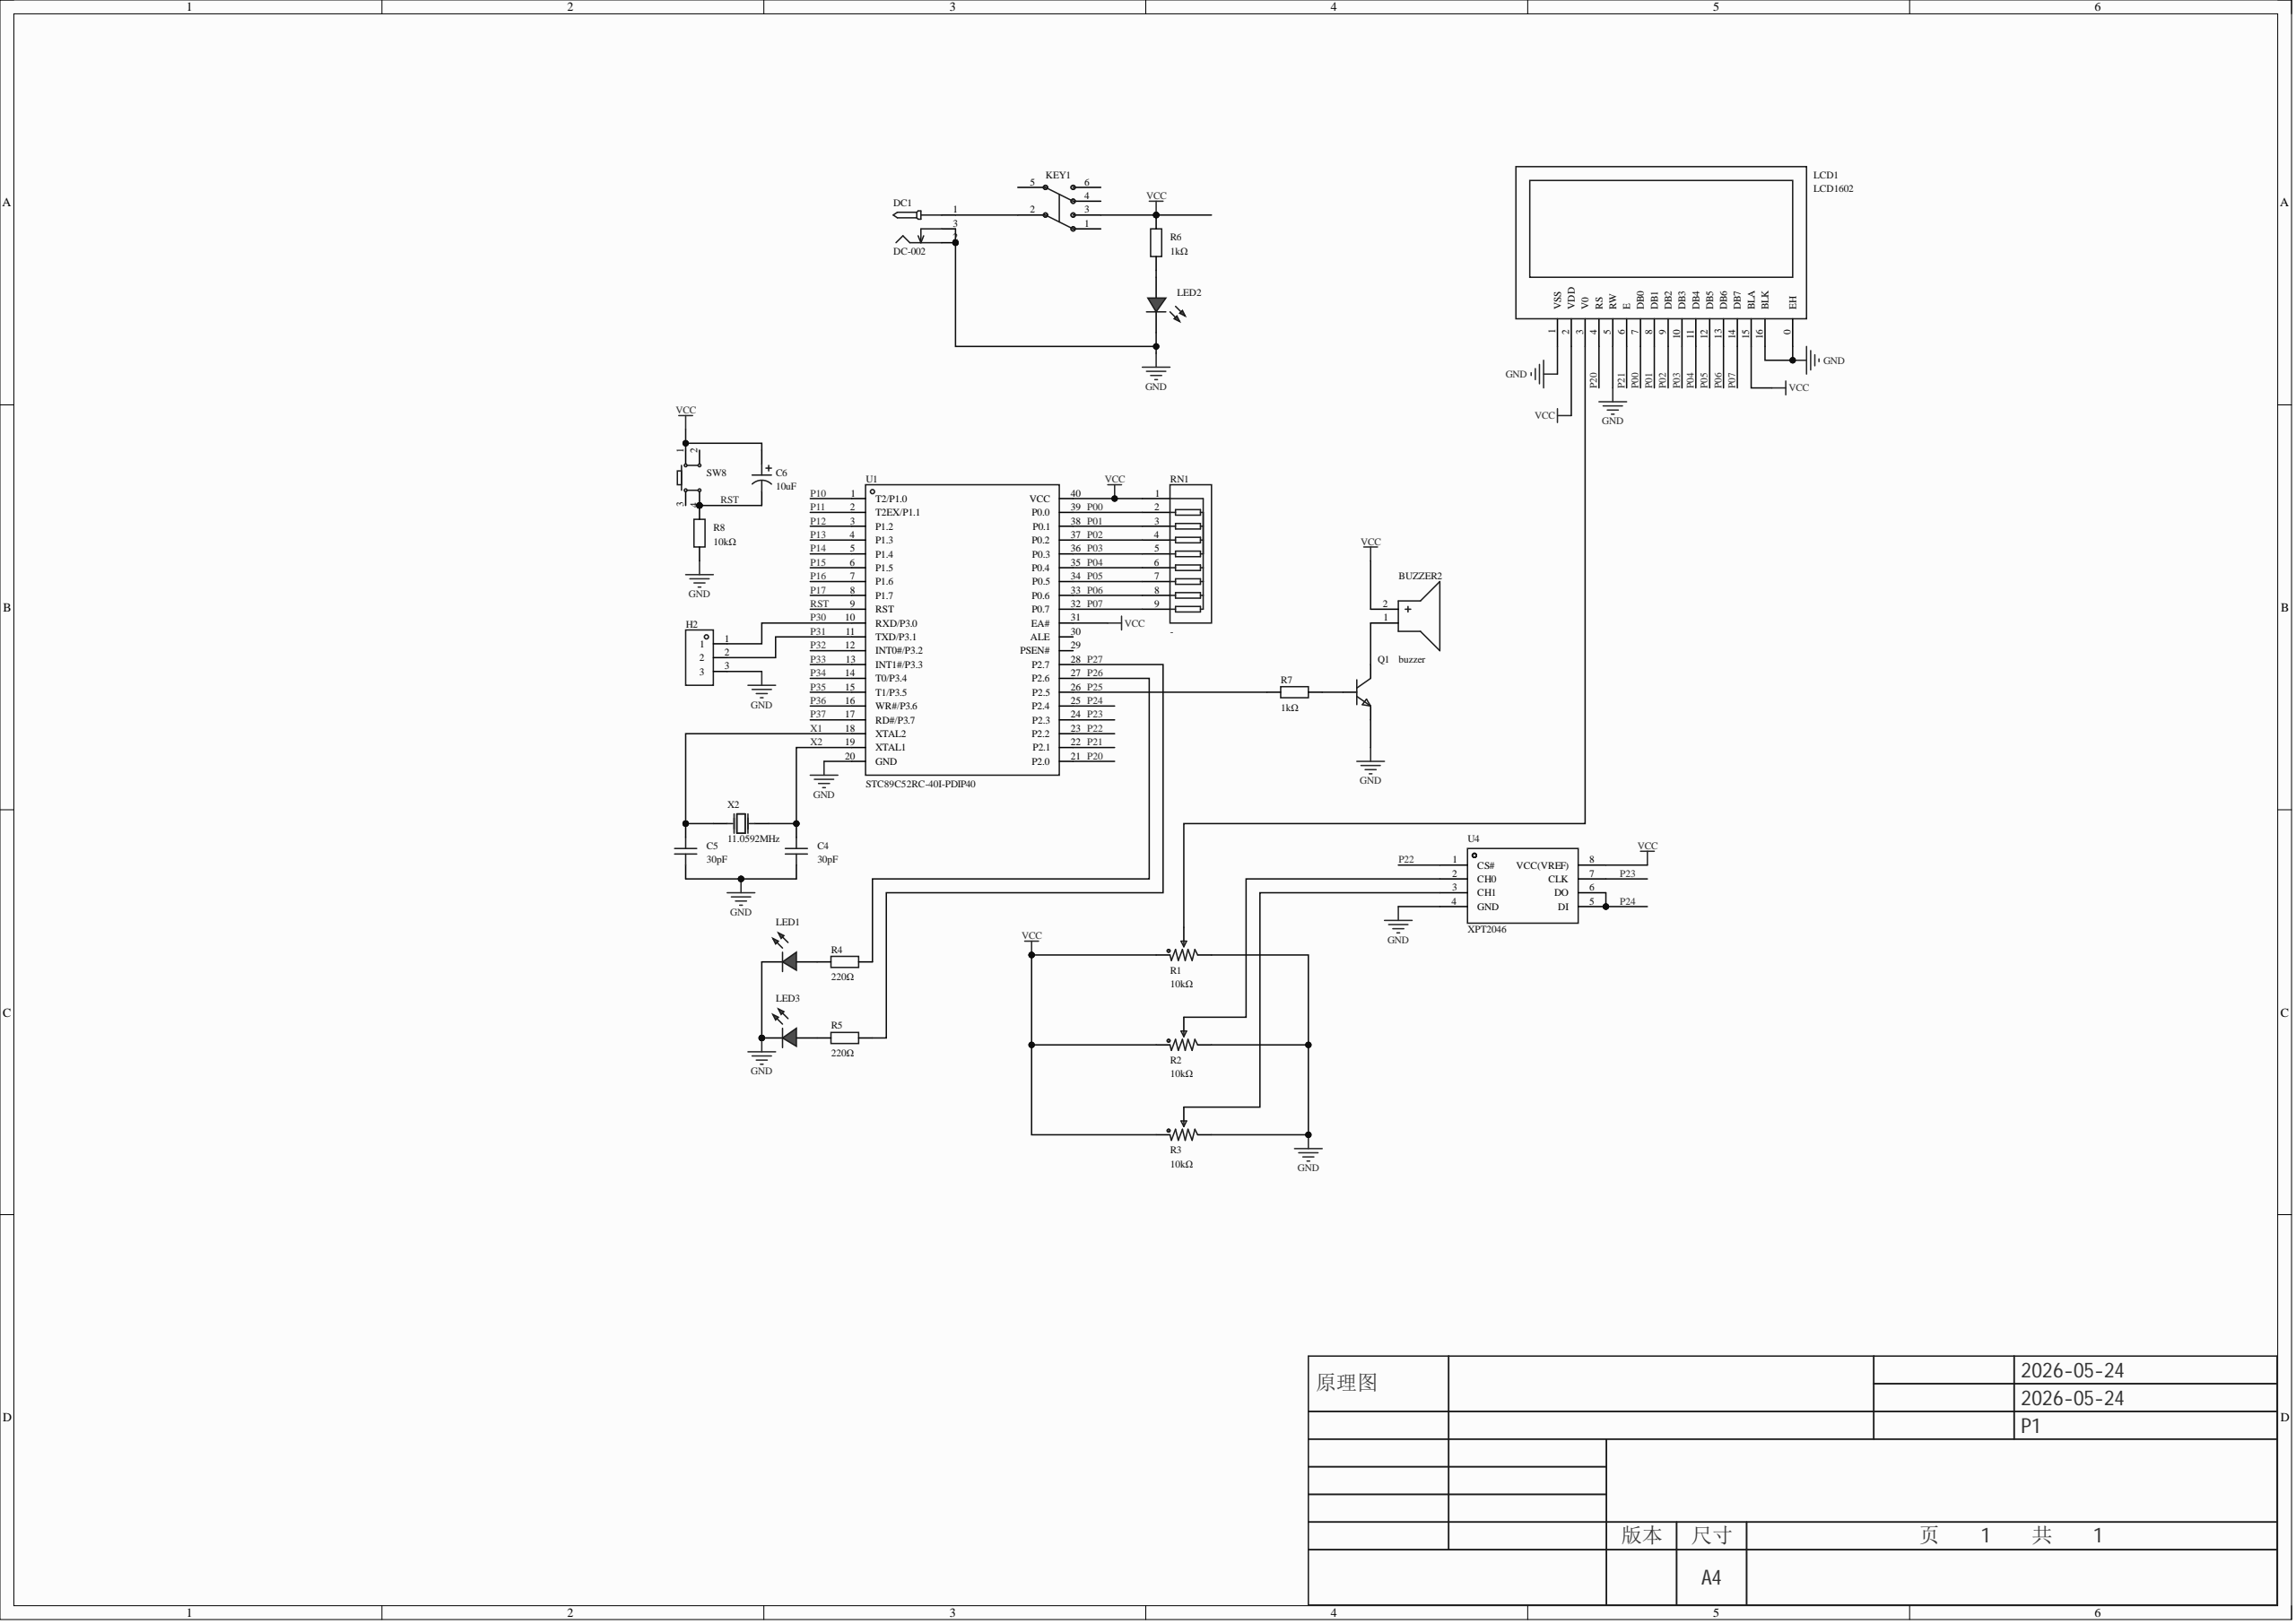Circuit board | Altium Designer | 25 parts | 32 nets
Bill of materials:
Comment,Description,Designator,Footprint,LibRef,Quantity
"buzzer","","BUZZER2","BUZ-TH_BD12.0-P6.00-D0.9-RD","buzzer","1"
"30pF","","C4, C5","CAP-TH_L3.8-W2.5-P2.54-D0.50","C315C300K3G5TA7301","2"
"10uF","","C6","CAP-TH_BD5.0-P2.00-D0.8-FD-10UF50VC110GL","10UF50VC110GL","1"
"DC-002","","DC1","DC-IN-TH_DC-3510","DC-002","1"
"","","H2","HDR-TH_3P-P2.54-V-M","HDR-M_2.54_1x3P","1"
"无自锁开关 8.5×8.5 无声","","KEY1","SW-TH_6P-L8.5-W8.5-P2.54","无自锁开关 8.5×8.5 无声","1"
"LCD1602","","LCD1","LCD1602","HS1602A","1"
"","","LED1, LED2, LED3","LED_TH-3mm","LED_TH-R_3mm","3"
"","","Q1","S8050_TO_92","S8050_TO_NPN","1"
"10kΩ","","R1, R2, R3","RES-ADJ-SMD_RM065-V1","RM065-103(10K)","3"
"220Ω","","R4, R5","Res_1/8W","Res_AXIAL-1/8W","2"
"1kΩ","","R6, R7","Res_1/8W","Res_AXIAL-1/8W","2"
"10kΩ","","R8","Res_1/8W","Res_AXIAL-1/8W","1"
"-","","RN1","RES-ARRAY-TH_9P-P2.54-D1.0","排阻 10 K 5%","1"
"","","SW8","SW-TH_4P-L6.0-W6.0-P4.50-LS6.5","Key_TH_6x6x6","1"
"STC89C52RC-40I-PDIP40","","U1","DIP-40_L52.0-W13.7-P2.54-LS15.2-BL","STC89C52RC-40I-PDIP40","1"
"XPT2046","","U4","DIP-8_L9.7-W6.4-P2.54-LS7.6-BL","ADC0832CCN","1"
"11.059MHz","","X2","OSC-TH_L11.1-W4.7-P4.88","9AC11059302060C3","1"
Netlist (Protel format):
[
BUZZER2
BUZ-TH_BD12.0-P6.00-D0.9-RD
buzzer



]
[
C4
CAP-TH_L3.8-W2.5-P2.54-D0.50
30pF



]
[
C5
CAP-TH_L3.8-W2.5-P2.54-D0.50
30pF



]
[
C6
CAP-TH_BD5.0-P2.00-D0.8-FD-10UF50VC110GL
10uF



]
[
DC1
DC-IN-TH_DC-3510
DC-002



]
[
H2
HDR-TH_3P-P2.54-V-M




]
[
KEY1
SW-TH_6P-L8.5-W8.5-P2.54
无自锁开关 8.5×8.5 无声



]
[
LCD1
LCD1602
LCD1602



]
[
LED1
LED_TH-3mm




]
[
LED2
LED_TH-3mm




]
[
LED3
LED_TH-3mm




]
[
Q1
S8050_TO_92




]
[
R1
RES-ADJ-SMD_RM065-V1
10kΩ



]
[
R2
RES-ADJ-SMD_RM065-V1
10kΩ



]
[
R3
RES-ADJ-SMD_RM065-V1
10kΩ



]
[
R4
Res_1/8W
220Ω



]
[
R5
Res_1/8W
220Ω



]
[
R6
Res_1/8W
1kΩ



]
[
R7
Res_1/8W
1kΩ



]
[
R8
Res_1/8W
10kΩ



]
[
RN1
RES-ARRAY-TH_9P-P2.54-D1.0
-



]
[
SW8
SW-TH_4P-L6.0-W6.0-P4.50-LS6.5




]
[
U1
DIP-40_L52.0-W13.7-P2.54-LS15.2-BL
STC89C52RC-40I-PDIP40



]
[
U4
DIP-8_L9.7-W6.4-P2.54-LS7.6-BL
XPT2046



]
[
X2
OSC-TH_L11.1-W4.7-P4.88
11.0592MHz



]
(
X2
C4-2
U1-19
X2-2
)
(
X1
C5-2
U1-18
X2-1
)
(
VCC
BUZZER2-2
C6-1
KEY1-3
LCD1-2
LCD1-15
R1-1
R2-1
R3-1
R6-2
RN1-1
SW8-1
U1-31
U1-40
U4-8
)
(
RST
C6-2
R8-2
SW8-4
U1-9
)
(
P31
H2-2
U1-11
)
(
P30
H2-1
U1-10
)
(
P27
R5-2
U1-28
)
(
P26
R4-2
U1-27
)
(
P25
R7-2
U1-26
)
(
P24
U1-25
U4-5
U4-6
)
(
P23
U1-24
U4-7
)
(
P22
U1-23
U4-1
)
(
P21
LCD1-6
U1-22
)
(
P20
LCD1-4
U1-21
)
(
P07
LCD1-14
RN1-9
U1-32
)
(
P06
LCD1-13
RN1-8
U1-33
)
(
P05
LCD1-12
RN1-7
U1-34
)
(
P04
LCD1-11
RN1-6
U1-35
)
(
P03
LCD1-10
RN1-5
U1-36
)
(
P02
LCD1-9
RN1-4
U1-37
)
(
P01
LCD1-8
RN1-3
U1-38
)
(
P00
LCD1-7
RN1-2
U1-39
)
(
NetR3_2
R3-2
U4-3
)
(
NetR2_2
R2-2
U4-2
)
(
NetQ1_2
Q1-2
R7-1
)
(
NetLED3_1
LED3-1
R5-1
)
(
NetLED2_1
LED2-1
R6-1
)
(
NetLED1_1
LED1-1
R4-1
)
(
NetLCD1_3
LCD1-3
R1-2
)
(
NetDC1_1
DC1-1
KEY1-2
)
(
NetBUZZER2_1
BUZZER2-1
Q1-3
)
(
GND
C4-1
C5-1
DC1-2
DC1-3
H2-3
LCD1-0
LCD1-1
LCD1-5
LCD1-16
LED1-2
LED2-2
LED3-2
Q1-1
R1-3
R2-3
R3-3
R8-1
U1-20
U4-4
)